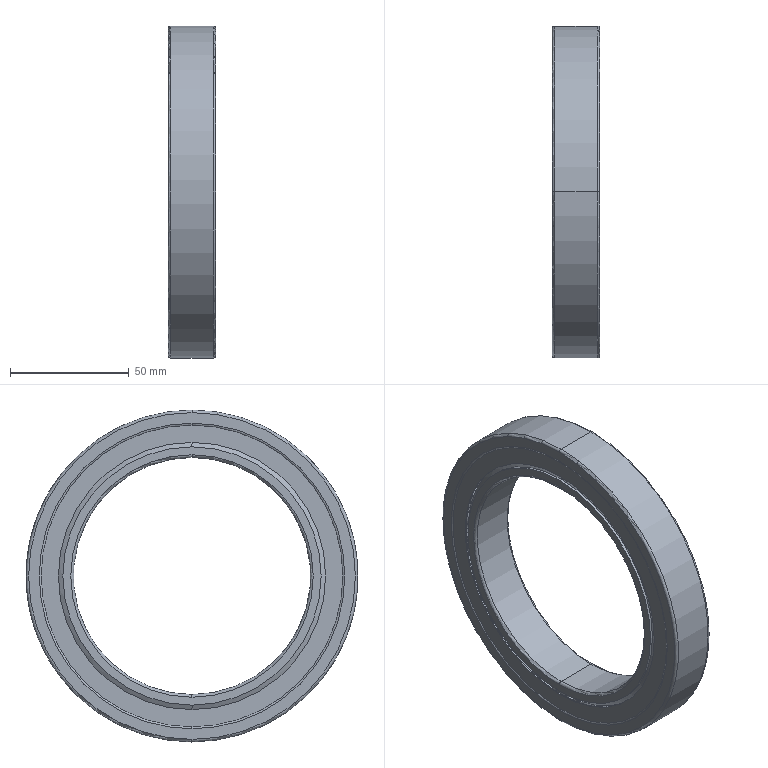Part | NX | features BREP 32 | 32 solids | 352 faces | box 20 x 140 x 140 mm | volume 112860 mm3 | cylinder 134 | sphere 124 | plane 68 | torus 22 | cone 4 | commonest cylinder face diameters 118 x59 122 x59 108.889 x4 113.333 x4 126.667 x4 100 x2